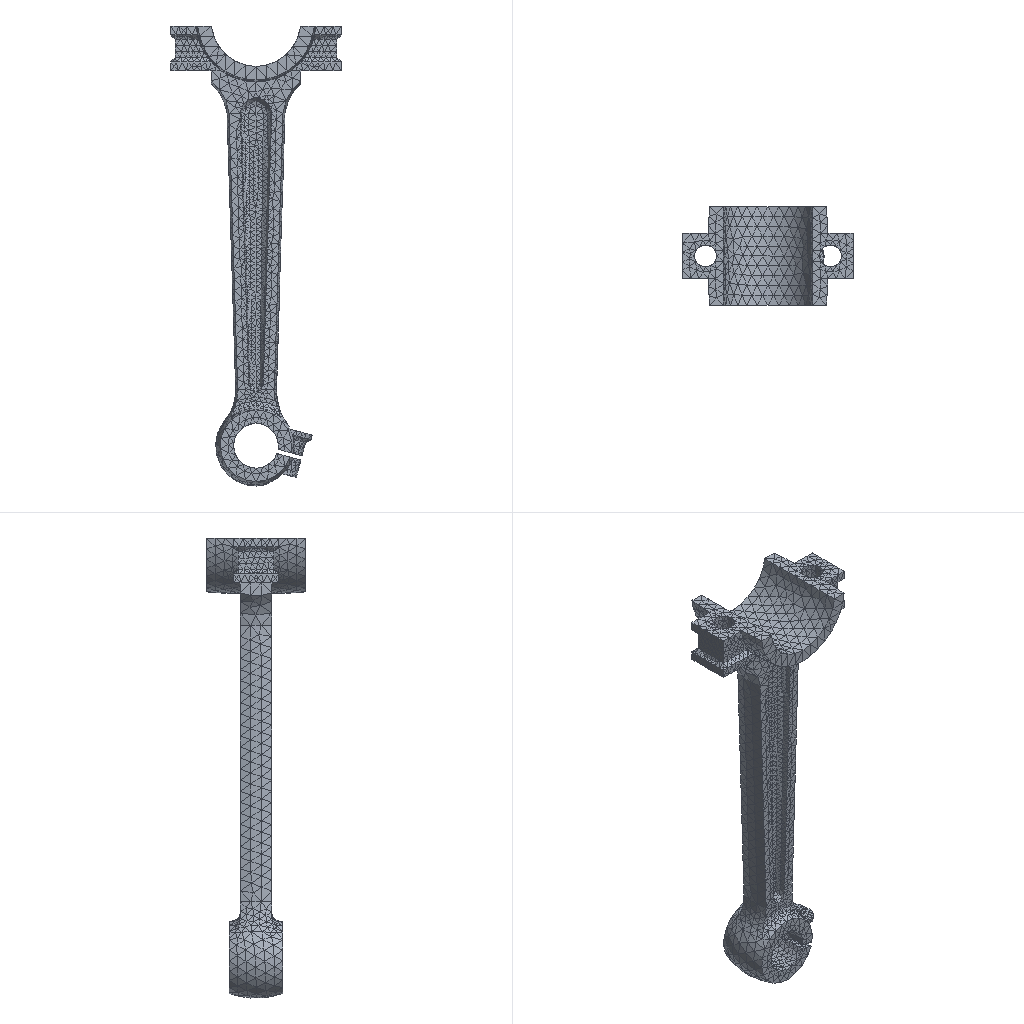Simulation study | nx simcenter
Set-up summary:
category,name,step,type,value,unit,region
solver,nx_nastran (Simcenter)
units,not stated in the deck,,not stated
analysis,deck,,static,static
analysis,solution,,SOL,101
load_step,SUBCASE 1,1,SUBCASE,SPC=1 LOAD=2
load_step,requested,,,1
mesh,nodes,,,23125
mesh,elements,,,12663
element_type,CTETRA,,solid,12663
load,nodal force total,,FX,0.0,model units
load,nodal force total,,FY,0.0,model units
load,nodal force total,,FZ,0.0,model units
load,load commands in deck,,count,236
bc,support commands in deck,,count,1278
analysis,NX solution 0,,Structural,SESTATIC 101 - Single Constraint
check,setup vs results,,match,every grid point's frame and coordinates and every element id; grid points of CTETRA elements
Nastran input file, long lists of numbers shortened:
$*$$$$$$$$$$$$$$$$$$$$$$$$$$$$$$$$$$$$$$$$$$$$$$$$$$$$$$$$$$$$$$$$$
$*
$*                    Simcenter v12.0.0.27 Translator
$*                    for NX Nastran version 12.0
$ (40 more lines like these left out)
ID,NASTRAN,有限元分析文件_fem1_sim1-solution_1
SOL 101
CEND
$*
$*$$$$$$$$$$$$$$$$$$$$$$$$$$$$$$$$$$$
$*
$* CASE CONTROL
$*
$*$$$$$$$$$$$$$$$$$$$$$$$$$$$$$$$$$$$
$*
ECHO = NONE
SPC = 1
OUTPUT
DISPLACEMENT(PLOT,REAL) = ALL
SPCFORCES(PLOT,REAL) = ALL
STRESS(PLOT,REAL,VONMISES,CENTER) = ALL
$*  Step: Subcase - Static Loads 1
SUBCASE 1
  LABEL = Subcase - Static Loads 1
  LOAD = 2
$*
$*$$$$$$$$$$$$$$$$$$$$$$$$$$$$$$$$$$$
$*
$* BULK DATA
$*
$*$$$$$$$$$$$$$$$$$$$$$$$$$$$$$$$$$$$
$*
BEGIN BULK
$*
$* PARAM CARDS
$*
PARAM      K6ROT100.0000
PARAM     OIBULK     YES
PARAM    OMACHPR     YES
PARAM       POST      -2
PARAM    POSTEXT     YES
PARAM    UNITSYS   MN-MM
$*
$* GRID CARDS
$*
GRID*                  1               02.1961173371E+017.6741330027E+00+
*       1.5013060735E+02               0
GRID*                  2               01.8965825825E+016.2645495868E+00+
*       1.5030954783E+02               0
$ (46246 more lines like these left out)
$*
$* ELEMENT CARDS
$*
$*  Mesh Collector: Solid(2)
$*  Mesh: 3d_mesh(1)
CTETRA         1       2   23083   21959       1       2   21960     723+
+            724     725     726     727
CTETRA         2       2   23046       3   23085       2     728     729+
+          21963     730     731     732
$ (25322 more lines like these left out)
$*
$* PROPERTY CARDS
$*
$*  Property: PSOLID2
PSOLID         2       1       0                           SMECH
$*
$* MATERIAL CARDS
$*
$*  Material: AISI_SS_304-Annealed::[REDACTED]::[1]
MAT1           11.9000+8        0.3000007.9000-61.6600-5
$*
$* LOAD AND CONSTRAINT CARDS
$*
$*  Constraint: Fixed(1)
SPC            1   12847  123456  0.0000
SPC            1   12848  123456  0.0000
SPC            1   12849  123456  0.0000
SPC            1   12850  123456  0.0000
$ (1274 more lines like these left out)
$*  Load: Pressure(1)
PLOAD4         2      59 2000.00                           21990   17613
PLOAD4         2     810 2000.00                           13944     439
PLOAD4         2    1178 2000.00                           14003      60
PLOAD4         2    1203 2000.00                           14005      59
$ (232 more lines like these left out)
ENDDATA ad8bba9f
Results summary:
result,analysis,,,static
result,last_loadstep,,,1
result,primary field,,,displacements
result,max displacement,,,0.02573,model units
result,reaction total,,FX,0.02579,model units
result,reaction total,,FY,-0.147,model units
result,reaction total,,FZ,3502355.5,model units
result,NX solution 0,,loadcases,1,mm